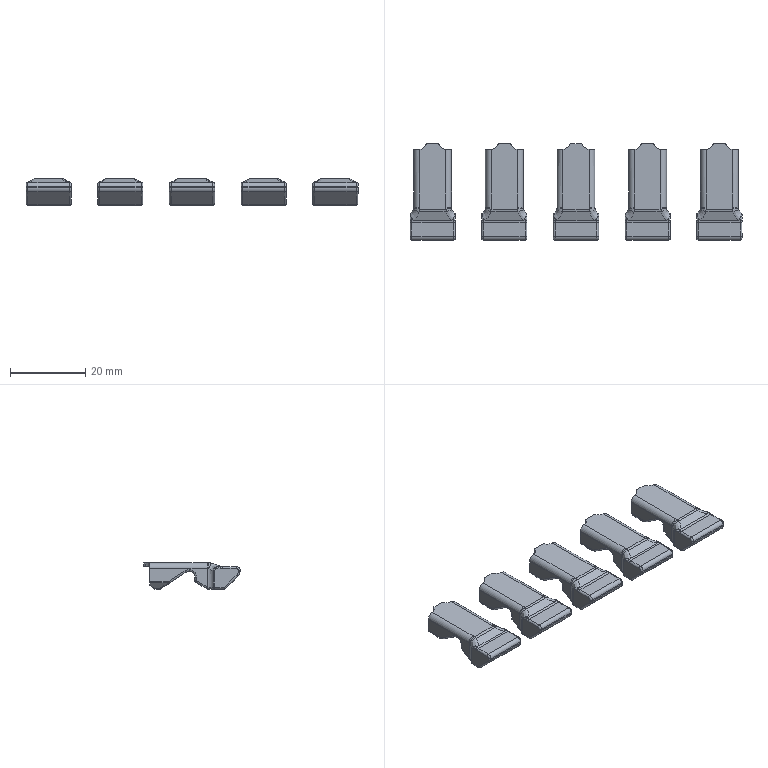NC program | NX | posted with a generic post | part box 88 x 25.5 x 7 mm
Lines 1 to 1151 of 11356:
N10 G17 G21 G94 G90
(FIXED_CONTOUR_COPY , TOOL : D4R0.5)
N12 T18 M6
N14 G54
N16 G17 G0 G90 X12.471 Y-7.984 S9500 M3
N18 G43 Z30. H18
N20 Z2.
N22 G94 G1 Z-2.898 F2500.
N24 X12.434 Y-7.987 Z-2.5
N26 X12.425 Z-2.401
N28 X12.353 Y-7.993 Z-2.4
N30 X12.313 Y-7.996 Z-2.305
N32 X12.265 Z-2.202
N34 X12.099 Z-2.032
N36 X12.03 Y-7.992 Z-1.974
N38 X11.941 Y-7.991 Z-1.95
N40 X11.702 Y-7.993 Z-1.909
N42 X8.531 Y-7.992 Z-1.899
N44 X7.995 Y-7.99 Z-1.883
N46 X7.831 Y-7.991 Z-1.878
N48 X7.738 Y-7.992 Z-1.869
N50 X7.342 Y-7.994 Z-1.807
N52 X7.216 Y-7.992 Z-1.79
N54 X6.945 Y-7.993 Z-1.788
N56 X6.828 Y-7.992 Z-1.808
N58 X6.549 Y-7.994 Z-1.891
N60 X6.318 Y-7.996 Z-2.026
N62 X6.139 Z-2.187
N64 X6.089 Y-7.995 Z-2.244
N66 X5.988 Y-7.993 Z-2.421
N68 X5.919 Y-7.99 Z-2.632
N70 X5.834 Y-7.987 Z-2.724
N72 Z-2.756
N74 X5.767 Y-7.984 Z-2.752
N76 X5.723 Y-7.979 Z-2.745
N78 X5.724 Z-2.721
N80 X5.756 Y-7.984 Z-2.651
N82 X5.761
N84 X5.827 Y-7.986 Z-2.584
N86 X5.875 Y-7.987 Z-2.447
N88 X5.992 Y-7.985 Z-2.214
N90 X6.153 Y-7.987 Z-2.039
N92 X6.218 Y-7.986 Z-1.981
N94 X6.337 Y-7.985 Z-1.899
N96 X6.4 Z-1.862
N98 X6.549 Y-7.983 Z-1.787
N100 X6.783 Y-7.981 Z-1.718
N102 X6.825 Y-7.98 Z-1.708
N104 X6.945 Y-7.981 Z-1.689
N106 X7.222 Z-1.69
N108 X7.354 Y-7.982 Z-1.709
N110 X7.751 Y-7.98 Z-1.77
N112 X7.995 Y-7.979 Z-1.793
N114 X8.135 Z-1.797
N116 X8.531 Y-7.98 Z-1.8
N118 X11.715 Y-7.981 Z-1.811
N120 X12.085 Y-7.983 Z-1.891
N122 X12.101 Y-7.984 Z-1.904
N124 X12.22 Y-7.987 Z-2.013
N126 X12.311 Z-2.107
N128 X12.407 Y-7.989 Z-2.271
N130 X12.487 Y-7.983 Z-2.322
N132 X12.495 Y-7.982 Z-2.33
N134 X12.521 Y-7.979 Z-2.479
N136 Z-2.5
N138 Z-2.479
N140 X12.516 Z-2.451
N142 X12.515 Z-2.298
N144 X12.495 Z-2.256
N146 X12.309 Z-1.988
N148 X12.114 Z-1.871
N150 X12.099 Z-1.864
N152 X11.702 Z-1.799
N154 X8.488
N156 X8.135 Z-1.797
N158 X7.995 Z-1.793
N160 X7.759 Z-1.769
N162 X7.738 Z-1.767
N164 X7.342 Z-1.687
N166 X6.945 Z-1.679
N168 X6.549 Z-1.759
N170 X6.338 Z-1.843
N172 X6.153 Z-1.953
N174 X6.134 Z-1.97
N176 X6.11 Z-1.995
N178 X5.911 Z-2.239
N180 X5.756 Z-2.486
N182 X5.729 Z-2.564
N184 X5.728 Z-2.712
N186 X5.724 Z-2.721
N188 X5.723 Z-2.745
N190 X5.656 Y-7.969 Z-2.735
N192 X5.661 Z-2.67
N194 X5.662 Z-2.565
N196 X5.756 Z-2.299
N198 X5.774 Z-2.27
N200 X5.797 Z-2.242
N202 X5.992 Z-2.029
N204 X6.153 Z-1.888
N206 X6.208 Z-1.854
N208 X6.34 Z-1.786
N210 X6.485 Z-1.735
N212 X6.549 Z-1.71
N214 X6.826 Z-1.661
N216 X6.945 Z-1.636
N218 X7.342 Z-1.647
N220 X7.738 Z-1.726
N222 X7.995 Z-1.757
N224 X8.135 Z-1.76
N226 X11.702
N228 X11.824 Z-1.78
N230 X12.099 Z-1.818
N232 X12.233 Z-1.877
N234 X12.308 Z-1.922
N236 X12.454 Z-2.045
N238 X12.495 Z-2.104
N240 X12.595 Z-2.315
N242 X12.596 Z-2.5
N244 X12.695 Y-7.956
N246 X12.694 Z-2.336
N248 X12.545 Z-2.058
N250 X12.495 Z-1.997
N252 X12.406 Z-1.922
N254 X12.334 Z-1.872
N256 X12.305 Z-1.855
N258 X12.144 Z-1.785
N260 X12.099 Z-1.769
N262 X12.007 Z-1.758
N264 X11.702 Z-1.716
N266 X8.135
N268 X7.995 Z-1.712
N270 X7.738 Z-1.68
N272 X7.342 Z-1.601
N274 X6.945 Z-1.591
N276 X6.549 Z-1.66
N278 X6.502 Z-1.674
N280 X6.342 Z-1.73
N282 X6.297 Z-1.75
N284 X6.153 Z-1.825
N286 X6.082 Z-1.875
N288 X5.898 Z-2.03
N290 X5.816 Z-2.103
N292 X5.756 Z-2.168
N294 X5.704 Z-2.261
N296 X5.601 Z-2.501
N298 X5.578 Z-2.566
N300 Z-2.588
N302 X5.568 Z-2.726
N304 X5.474 Y-7.935 Z-2.735
N306 X5.48 Z-2.583
N308 X5.561 Z-2.353
N310 X5.611 Z-2.236
N312 X5.639 Z-2.186
N314 X5.756 Z-2.042
N316 X5.895 Z-1.925
N318 X6.153 Z-1.742
N320 X6.18 Z-1.728
N322 X6.345 Z-1.656
N324 X6.549 Z-1.591
N326 X6.945 Z-1.527
N328 X7.342 Z-1.533
N330 X7.738 Z-1.61
N332 X7.995 Z-1.646
N334 X8.135 Z-1.649
N336 X11.702 Z-1.65
N338 X12.099 Z-1.698
N340 X12.265 Z-1.758
N342 X12.301 Z-1.774
N344 X12.424 Z-1.845
N346 X12.495 Z-1.895
N348 X12.548 Z-1.941
N350 X12.621 Z-2.018
N352 X12.648 Z-2.051
N354 X12.689 Z-2.128
N356 X12.757 Z-2.276
N358 X12.788 Z-2.36
N360 X12.789 Z-2.5
N362 X12.886 Y-7.914
N364 Z-2.385
N366 X12.82 Z-2.213
N368 X12.762 Z-2.083
N370 X12.733 Z-2.038
N372 X12.682 Z-1.973
N374 X12.626 Z-1.913
N376 X12.543 Z-1.842
N378 X12.495 Z-1.81
N380 X12.342 Z-1.729
N382 X12.297 Z-1.711
N384 X12.252 Z-1.699
N386 X12.099 Z-1.644
N388 X12. Z-1.635
N390 X11.702 Z-1.6
N392 X8.135 Y-7.913
N394 X7.995 Z-1.596
N396 X7.802 Z-1.569
N398 X7.342 Z-1.481
N400 X6.945 Z-1.476
N402 X6.648 Z-1.524
N404 X6.549 Z-1.538
N406 X6.397 Z-1.585
N408 X6.348 Z-1.598
N410 X6.297 Z-1.615
N412 X6.153 Z-1.678
N414 X6.063 Z-1.728
N416 X5.756 Z-1.94
N418 X5.743 Z-1.952
N420 X5.705 Z-1.99
N422 X5.567 Z-2.16
N424 X5.527 Z-2.22
N426 X5.506 Z-2.262
N428 X5.385 Z-2.603
N430 X5.383 Z-2.744
N432 X5.36 Y-7.908 Z-2.746
N434 X5.298 Y-7.888 Z-2.752
N436 Z-2.651
N438 X5.3 Z-2.622
N440 X5.36 Z-2.39
N442 X5.375 Z-2.347
N444 X5.443 Z-2.211
N446 X5.518 Z-2.099
N448 X5.549 Z-2.057
N450 X5.688 Z-1.912
N452 X5.756 Z-1.855
N454 X5.927 Z-1.736
N456 X6.153 Z-1.612
N458 X6.225 Z-1.581
N460 X6.352 Z-1.536
N462 X6.473 Z-1.505
N464 X6.549 Z-1.481
N466 X6.797 Z-1.447
N468 X6.945 Z-1.423
N470 X7.342 Z-1.428
N472 X7.59 Z-1.473
N474 X7.899 Z-1.531
N476 X7.995 Z-1.545
N478 X8.135 Z-1.549
N480 X11.702
N482 X11.851 Z-1.567
N484 X12.099 Z-1.588
N486 X12.175 Z-1.616
N488 X12.292 Z-1.648
N490 X12.408 Z-1.695
N492 X12.495 Z-1.741
N494 X12.56 Z-1.779
N496 X12.674 Z-1.859
N498 X12.707 Z-1.887
N500 X12.748 Z-1.93
N502 X12.818 Z-2.019
N504 X12.894 Z-2.142
N506 X12.968 Z-2.383
N508 X12.969 Z-2.5
N510 X13.064 Y-7.858
N512 X13.063 Z-2.379
N514 X13.044 Z-2.316
N516 X12.975 Z-2.122
N518 X12.923 Z-2.018
N520 X12.892 Z-1.975
N522 X12.788 Z-1.866
N524 X12.664 Z-1.763
N526 X12.624 Z-1.735
N528 X12.487 Z-1.655
N530 X12.287 Z-1.576
N532 X12.099 Z-1.525
N534 X11.702 Z-1.492
N536 X8.135 Z-1.491
N538 X7.995 Z-1.486
N540 X7.342 Z-1.369
N542 X6.945 Z-1.364
N544 X6.549 Z-1.418
N546 X6.357 Z-1.466
N548 X6.153 Z-1.537
N550 X6.126 Z-1.55
N552 X5.768 Z-1.745
N554 X5.756 Z-1.753
N556 X5.624 Z-1.865
N558 X5.582 Z-1.909
N560 X5.468 Z-2.033
N562 X5.36 Z-2.182
N564 X5.342 Z-2.212
N566 X5.286 Z-2.343
N568 X5.209 Z-2.642
N570 X5.204 Z-2.717
N572 Z-2.762
N574 X5.137 Y-7.837 Z-2.763
N576 X5.109 Y-7.825
N578 X5.114 Z-2.656
N580 X5.142 Z-2.533
N582 X5.196 Z-2.326
N584 X5.215 Z-2.282
N586 X5.268 Z-2.18
N588 X5.36 Z-2.033
N590 X5.379 Z-2.006
N592 X5.433 Z-1.948
N594 X5.556 Z-1.828
N596 X5.591 Z-1.796
N598 X5.69 Z-1.72
N600 X5.756 Z-1.674
N602 X5.941 Z-1.573
N604 X6.153 Y-7.826 Z-1.476
N606 X6.272 Z-1.439
N608 X6.362 Z-1.408
N610 X6.464 Z-1.386
N612 X6.549 Z-1.364
N614 X6.771 Z-1.339
N616 X6.945 Z-1.315
N618 X7.342 Z-1.321
N620 X7.516 Z-1.352
N622 X7.738 Z-1.384
N624 X7.995 Z-1.434
N626 X8.073 Z-1.44
N628 X8.135 Z-1.442
N630 X11.702
N632 X11.877 Z-1.457
N634 X12.099 Z-1.472
N636 X12.183 Z-1.496
N638 X12.28 Z-1.516
N640 X12.385 Z-1.556
N642 X12.495 Z-1.591
N644 X12.557 Z-1.622
N646 X12.653 Z-1.673
N648 X12.693 Z-1.699
N650 X12.838 Z-1.811
N652 X12.878 Z-1.844
N654 X12.892 Z-1.858
N656 X12.985 Z-1.977
N658 X13.054 Z-2.08
N660 X13.064 Z-2.1
N662 X13.088 Z-2.168
N664 X13.141 Z-2.34
N666 X13.153 Z-2.384
N668 Z-2.5
N670 X13.246 Y-7.788
N672 Z-2.397
N674 X13.214 Z-2.278
N676 X13.173 Z-2.147
N678 X13.152 Z-2.096
N680 X13.071 Z-1.953
N682 X12.945 Z-1.81
N684 X12.892 Z-1.766
N686 X12.769 Z-1.672
N688 X12.634 Z-1.586
N690 X12.495 Z-1.519
N692 X12.273 Z-1.451
N694 X12.099 Z-1.416
N696 X11.702 Z-1.388
N698 X8.135
N700 X8. Z-1.379
N702 X7.738 Z-1.325
N704 X7.342 Z-1.268
N706 X6.945 Z-1.261
N708 X6.549 Z-1.307
N710 X6.341 Z-1.353
N712 X6.13 Z-1.418
N714 X5.756 Z-1.59
N716 X5.609 Z-1.688
N718 X5.48 Z-1.804
N720 X5.326 Z-1.953
N722 X5.302 Z-1.982
N724 X5.196 Z-2.128
N726 X5.177 Z-2.158
N728 X5.16 Z-2.192
N730 X5.102 Z-2.322
N732 X5.065 Z-2.466
N734 X5.023 Z-2.649
N736 X5.021 Z-2.763
N738 X4.931 Y-7.749
N740 X4.932 Z-2.666
N742 X4.948 Z-2.569
N744 X4.963 Z-2.515
N746 X5.011 Z-2.332
N748 X5.089 Z-2.157
N750 X5.162 Z-2.044
N752 X5.178 Z-2.025
N754 X5.226 Z-1.959
N756 X5.283 Z-1.891
N758 X5.401 Z-1.779
N760 X5.51 Z-1.681
N762 X5.612 Z-1.611
N764 X5.701 Z-1.561
N766 X5.756 Z-1.525
N768 X6.014 Z-1.405
N770 X6.153 Z-1.356
N772 X6.355 Z-1.298
N774 X6.549 Z-1.259
N776 X6.945 Z-1.216
N778 X7.342 Z-1.22
N780 X7.738 Z-1.274
N782 X8.025 Z-1.335
N784 X8.135 Z-1.341
N786 X11.702
N788 X12.099 Z-1.368
N790 X12.266 Z-1.398
N792 X12.428 Z-1.446
N794 X12.495 Z-1.466
N796 X12.58 Z-1.497
N798 X12.674 Z-1.541
N800 X12.801 Z-1.613
N802 X12.85 Z-1.644
N804 X13.01 Z-1.773
N806 X13.083 Z-1.854
N808 X13.149 Z-1.933
N810 X13.18 Z-1.984
N812 X13.242 Z-2.098
N814 X13.291 Z-2.217
N816 X13.322 Z-2.345
N818 X13.334 Z-2.42
N820 Z-2.5
N822 X13.375 Y-7.729
N824 X13.419 Y-7.705
N826 Z-2.424
N828 X13.402 Z-2.317
N830 X13.391 Z-2.27
N832 X13.374 Z-2.213
N834 X13.34 Z-2.119
N836 X13.288 Z-2.01
N838 X13.247 Z-1.934
N840 X13.133 Z-1.791
N842 X13.109 Z-1.767
N844 X13.069 Z-1.732
N846 X12.954 Z-1.638
N848 X12.892 Z-1.594
N850 X12.742 Z-1.51
N852 X12.653 Z-1.469
N854 X12.543 Z-1.431
N856 X12.495 Z-1.411
N858 X12.355 Z-1.369
N860 X12.306 Z-1.357
N862 X12.249 Z-1.348
N864 X12.222 Z-1.342
N866 X12.099 Z-1.32
N868 X11.702 Z-1.294
N870 X8.098 Z-1.293
N872 X8.044 Z-1.288
N874 X7.738 Z-1.224
N876 X7.342 Z-1.172
N878 X6.945 Z-1.169
N880 X6.549 Z-1.209
N882 X6.302 Z-1.259
N884 X6.153 Z-1.3
N886 X5.906 Z-1.388
N888 X5.756 Z-1.458
N890 X5.554 Z-1.574
N892 X5.435 Z-1.655
N894 X5.294 Z-1.781
N896 X5.217 Z-1.866
N898 X5.166 Z-1.914
N900 X5.115 Z-1.974
N902 X5.004 Z-2.146
N904 X4.924 Z-2.33
N906 X4.885 Z-2.459
N908 X4.847 Z-2.688
N910 X4.844 Z-2.763
N912 X4.761 Y-7.657
N914 X4.765 Z-2.671
N916 X4.805 Z-2.447
N918 X4.845 Z-2.314
N920 X4.927 Z-2.129
N922 X5.02 Z-1.978
N924 X5.078 Z-1.906
N926 X5.165 Z-1.811
N928 X5.387 Z-1.61
N930 X5.431 Z-1.581
N932 X5.756 Z-1.394
N934 X5.811 Z-1.368
N936 X6.009 Z-1.301
N938 X6.153 Z-1.247
N940 X6.207 Z-1.232
N942 X6.549 Z-1.162
N944 X6.945 Z-1.124
N946 X7.342 Z-1.128
N948 X7.451 Z-1.142
N950 X7.738 Z-1.177
N952 X8.056 Z-1.241
N954 X8.1 Z-1.248
N956 X8.531 Z-1.251
N958 X11.702
N960 X12.099 Z-1.276
N962 X12.157 Z-1.287
N964 X12.3 Z-1.305
N966 X12.444 Z-1.34
N968 X12.495 Z-1.356
N970 X12.639 Z-1.414
N972 X12.718 Z-1.442
N974 X12.837 Z-1.494
N976 X12.892 Z-1.525
N978 X13.078 Z-1.654
N980 X13.165 Z-1.728
N982 X13.227 Z-1.789
N984 X13.288 Z-1.863
N986 X13.325 Z-1.913
N988 X13.35 Z-1.956
N990 X13.373 Z-2.013
N992 X13.442 Z-2.157
N994 X13.465 Z-2.226
N996 X13.499 Z-2.368
N998 X13.504 Z-2.4
N1000 Z-2.5
N1002 X13.555 Y-7.628
N1004 X13.585 Y-7.608
N1006 Z-2.392
N1008 X13.544 Z-2.198
N1010 X13.522 Z-2.132
N1012 X13.486 Z-2.046
N1014 X13.406 Z-1.909
N1016 X13.349 Z-1.832
N1018 X13.309 Z-1.783
N1020 X13.179 Z-1.655
N1022 X13.136 Z-1.622
N1024 X12.935 Z-1.483
N1026 X12.892 Z-1.46
N1028 X12.786 Z-1.414
N1030 X12.737 Z-1.397
N1032 X12.582 Z-1.334
N1034 X12.495 Z-1.305
N1036 X12.449 Z-1.296
N1038 X12.294 Z-1.258
N1040 X12.099 Z-1.233
N1042 X11.702 Z-1.21
N1044 X8.135 Z-1.209
N1046 X8.118 Z-1.208
N1048 X7.738 Z-1.132
N1050 X7.651 Z-1.124
N1052 X7.342 Z-1.087
N1054 X6.945 Z-1.083
N1056 X6.549 Z-1.118
N1058 X6.24 Z-1.182
N1060 X6.153 Z-1.197
N1062 X6.066 Z-1.225
N1064 X5.911 Z-1.283
N1066 X5.756 Z-1.334
N1068 X5.669 Z-1.377
N1070 X5.36 Z-1.555
N1072 X5.311 Z-1.59
N1074 X5.063 Z-1.817
N1076 X4.94 Z-1.97
N1078 X4.904 Z-2.023
N1080 X4.847 Z-2.118
N1082 X4.765 Z-2.298
N1084 X4.724 Z-2.438
N1086 X4.684 Z-2.669
N1088 X4.681 Z-2.763
N1090 X4.597 Y-7.554
N1092 X4.6 Z-2.685
N1094 X4.639 Z-2.447
N1096 X4.679 Z-2.304
N1098 X4.759 Z-2.109
N1100 X4.883 Z-1.928
N1102 X4.993 Z-1.787
N1104 X5.19 Z-1.604
N1106 X5.293 Z-1.536
N1108 X5.36 Z-1.482
N1110 X5.452 Z-1.429
N1112 X5.756 Z-1.278
N1114 X5.849 Z-1.245
N1116 X6.001 Z-1.199
N1118 X6.153 Z-1.149
N1120 X6.456 Z-1.095
N1122 X6.549 Z-1.076
N1124 X6.945 Z-1.044
N1126 X7.342 Z-1.048
N1128 X7.435 Z-1.059
N1130 X7.738 Z-1.088
N1132 X8.145 Z-1.168
N1134 X8.531 Z-1.17
N1136 X11.702
N1138 X12.099 Z-1.191
N1140 X12.288 Z-1.213
N1142 X12.334 Z-1.224
N1144 X12.495 Z-1.258
N1146 X12.799 Z-1.359
N1148 X12.892 Z-1.397
N1150 X13.043 Z-1.477
N1152 X13.104 Z-1.519
N1154 X13.255 Z-1.634
N1156 X13.362 Z-1.741
N1158 X13.493 Z-1.902
N1160 X13.584 Z-2.08
N1162 X13.642 Z-2.254
N1164 X13.664 Z-2.366
N1166 X13.669 Z-2.395
N1168 Z-2.5
N1170 X13.684 Y-7.544
N1172 X13.742 Y-7.498
N1174 Z-2.403
N1176 X13.723 Z-2.268
N1178 X13.684 Z-2.132
N1180 X13.674 Z-2.1
N1182 X13.588 Z-1.931
N1184 X13.557 Z-1.879
N1186 X13.417 Z-1.697
N1188 X13.389 Z-1.669
N1190 X13.288 Z-1.581
N1192 X13.156 Z-1.481
N1194 X13.07 Z-1.432
N1196 X12.938 Z-1.362
N1198 X12.892 Z-1.34
N1200 X12.628 Z-1.252
N1202 X12.495 Z-1.214
N1204 X12.355 Z-1.185
N1206 X12.281 Z-1.174
N1208 X12.099 Z-1.155
N1210 X11.702 Z-1.135
N1212 X8.283
N1214 X8.177 Z-1.136
N1216 X8.074 Z-1.114
N1218 X7.738 Z-1.05
N1220 X7.342 Z-1.013
N1222 X6.945 Z-1.009
N1224 X6.549 Z-1.039
N1226 X6.286 Z-1.086
N1228 X6.153 Z-1.107
N1230 X6.02 Z-1.143
N1232 X5.888 Z-1.187
N1234 X5.756 Z-1.227
N1236 X5.623 Z-1.287
N1238 X5.36 Z-1.417
N1240 X5.301 Z-1.453
N1242 X5.243 Z-1.499
N1244 X5.154 Z-1.559
N1246 X5.079 Z-1.617
N1248 X4.933 Z-1.756
N1250 X4.855 Y-7.497 Z-1.842
N1252 X4.823 Z-1.884
N1254 X4.799 Z-1.919
N1256 X4.67 Z-2.134
N1258 X4.59 Z-2.317
N1260 X4.567 Z-2.399
N1262 X4.553 Z-2.46
N1264 X4.524 Z-2.689
N1266 X4.522 Z-2.763
N1268 X4.446 Y-7.436
N1270 X4.448 Z-2.687
N1272 X4.455 Z-2.612
N1274 X4.472 Z-2.486
N1276 X4.509 Z-2.328
N1278 X4.571 Z-2.162
N1280 X4.732 Z-1.895
N1282 X4.763 Z-1.852
N1284 X4.833 Z-1.767
N1286 X4.875 Z-1.721
N1288 X4.97 Z-1.629
N1290 X5.192 Z-1.456
N1292 X5.36 Z-1.354
N1294 X5.661 Z-1.217
N1296 X5.756 Z-1.176
N1298 X6.057 Z-1.09
N1300 X6.153 Z-1.066
N1302 X6.549 Z-1.002
N1304 X6.945 Z-0.975
N1306 X7.342 Z-0.977
N1308 X7.738 Z-1.013
N1310 X8.135 Z-1.087
N1312 X8.211 Z-1.107
N1314 X8.516 Z-1.102
N1316 X11.702
N1318 X12.099 Z-1.121
N1320 X12.273 Z-1.138
N1322 X12.495 Z-1.171
N1324 X12.892 Z-1.285
N1326 X13.033 Z-1.352
N1328 X13.185 Z-1.437
N1330 X13.288 Z-1.5
N1332 X13.394 Z-1.591
N1334 X13.48 Z-1.67
N1336 X13.555 Z-1.759
N1338 X13.627 Z-1.853
N1340 X13.687 Z-1.955
N1342 X13.753 Z-2.105
N1344 X13.794 Z-2.25
N1346 X13.819 Z-2.413
N1348 Z-2.5
N1350 X13.897 Y-7.373
N1352 X13.896 Z-2.415
N1354 X13.867 Z-2.231
N1356 X13.831 Z-2.109
N1358 X13.765 Z-1.957
N1360 X13.7 Z-1.834
N1362 X13.544 Z-1.647
N1364 X13.471 Z-1.584
N1366 X13.426 Z-1.542
N1368 X13.306 Z-1.448
N1370 X13.247 Z-1.412
N1372 X13.066 Z-1.313
N1374 X12.996 Z-1.284
N1376 X12.939 Z-1.258
N1378 X12.774 Z-1.208
N1380 X12.612 Z-1.162
N1382 X12.495 Z-1.136
N1384 X12.265 Z-1.105
N1386 X12.099 Z-1.09
N1388 X11.937 Z-1.083
N1390 X11.702 Z-1.075
N1392 X8.375
N1394 X8.245 Z-1.078
N1396 X8.135 Z-1.05
N1398 X8.049 Z-1.032
N1400 X7.856 Z-0.997
N1402 X7.738 Z-0.982
N1404 X7.577 Z-0.967
N1406 X7.342 Z-0.95
N1408 X6.945 Z-0.947
N1410 X6.711 Z-0.961
N1412 X6.549 Z-0.972
N1414 X6.432 Z-0.985
N1416 X6.153 Z-1.03
N1418 X6.035 Z-1.055
N1420 X5.756 Z-1.133
N1422 X5.639 Z-1.174
N1424 X5.36 Z-1.3
N1426 X5.284 Z-1.341
N1428 X5.171 Z-1.409
N1430 X5.054 Z-1.491
N1432 X4.963 Z-1.561
N1434 X4.921 Z-1.597
N1436 X4.81 Z-1.7
N1438 X4.704 Z-1.825
N1440 X4.632 Z-1.926
N1442 X4.567 Z-2.033
N1444 X4.494 Z-2.171
N1446 X4.432 Z-2.338
N1448 X4.39 Z-2.512
N1450 X4.371 Z-2.686
N1452 X4.369 Z-2.763
N1454 X4.32 Y-7.333
N1456 X4.295 Y-7.308
N1458 X4.297 Z-2.687
N1460 X4.314 Z-2.525
N1462 X4.363 Z-2.331
N1464 X4.423 Z-2.167
N1466 X4.549 Z-1.932
N1468 X4.642 Z-1.802
N1470 X4.741 Z-1.69
N1472 X4.827 Z-1.606
N1474 X4.876 Z-1.563
N1476 X4.963 Z-1.49
N1478 X5.038 Z-1.437
N1480 X5.137 Z-1.371
N1482 X5.199 Z-1.335
N1484 X5.348 Z-1.254
N1486 X5.546 Z-1.166
N1488 X5.732 Z-1.1
N1490 X5.93 Z-1.044
N1492 X6.153 Z-0.998
N1494 X6.326 Z-0.97
N1496 X6.549 Z-0.944
N1498 X6.889 Z-0.926
N1500 X7.043 Z-0.924
N1502 X7.342 Z-0.926
N1504 X7.738 Z-0.954
N1506 X8.008 Z-0.989
N1508 X8.178 Z-1.025
N1510 X8.291 Z-1.052
N1512 X11.754 Z-1.053
N1514 X12.125 Z-1.066
N1516 X12.381 Z-1.09
N1518 X12.553 Z-1.114
N1520 X12.702 Z-1.147
N1522 X12.892 Z-1.204
N1524 X12.998 Z-1.238
N1526 X13.139 Z-1.298
N1528 X13.288 Z-1.378
N1530 X13.339 Z-1.409
N1532 X13.509 Z-1.54
N1534 X13.607 Z-1.626
N1536 X13.714 Z-1.755
N1538 X13.771 Z-1.83
N1540 X13.837 Z-1.951
N1542 X13.852 Z-1.983
N1544 X13.904 Z-2.103
N1546 X13.938 Z-2.213
N1548 X13.95 Z-2.281
N1550 X13.972 Z-2.419
N1552 X13.973 Z-2.5
N1554 X14.044 Y-7.238
N1556 X14.042 Z-2.412
N1558 X14.035 Z-2.36
N1560 X14.005 Z-2.197
N1562 X13.969 Z-2.08
N1564 X13.899 Z-1.933
N1566 X13.831 Z-1.811
N1568 X13.679 Z-1.619
N1570 X13.568 Z-1.516
N1572 X13.397 Z-1.389
N1574 X13.279 Z-1.319
N1576 X13.184 Z-1.274
N1578 X13.072 Z-1.228
N1580 X13.018 Z-1.211
N1582 X12.892 Z-1.167
N1584 X12.719 Z-1.114
N1586 X12.59 Z-1.094
N1588 X12.41 Z-1.069
N1590 X12.2 Z-1.051
N1592 X12.099 Z-1.044
N1594 X11.903 Z-1.038
N1596 X11.426 Z-1.033
N1598 X8.927
N1600 X8.527 Z-1.031
N1602 X8.466 Z-1.033
N1604 X8.359
N1606 X8.302 Z-1.02
N1608 X8.214 Z-1.005
N1610 X8.059 Z-0.971
N1612 X7.964 Z-0.958
N1614 X7.87 Z-0.95
N1616 X7.738 Z-0.933
N1618 X7.324 Z-0.905
N1620 X7.134 Z-0.907
N1622 X6.945 Z-0.906
N1624 X6.729 Z-0.913
N1626 X6.549 Z-0.921
N1628 X6.256 Z-0.954
N1630 X6.153 Z-0.971
N1632 X5.964 Z-1.007
N1634 X5.86 Z-1.029
N1636 X5.662 Z-1.085
N1638 X5.511 Z-1.138
N1640 X5.463 Z-1.156
N1642 X5.313 Z-1.223
N1644 X5.218 Z-1.271
N1646 X5.171 Z-1.3
N1648 X5.067 Z-1.358
N1650 X4.963 Z-1.422
N1652 X4.797 Z-1.558
N1654 X4.671 Z-1.679
N1656 X4.567 Z-1.793
N1658 X4.52 Z-1.867
N1660 X4.473 Z-1.932
N1662 X4.361 Z-2.141
N1664 X4.305 Z-2.291
N1666 X4.282 Z-2.371
N1668 X4.247 Z-2.514
N1670 X4.227 Z-2.693
N1672 X4.226 Z-2.763
N1674 X4.158 Y-7.167
N1676 Z-2.697
N1678 X4.179 Z-2.502
N1680 X4.205 Z-2.39
N1682 X4.247 Z-2.251
N1684 X4.298 Z-2.115
N1686 X4.338 Z-2.038
N1688 X4.403 Z-1.921
N1690 X4.448 Z-1.855
N1692 X4.484 Z-1.808
N1694 X4.5 Z-1.783
N1696 X4.55 Z-1.721
N1698 X4.615 Z-1.652
N1700 X4.726 Z-1.546
N1702 X4.83 Z-1.459
N1704 X4.93 Z-1.385
N1706 X5.111 Z-1.275
N1708 X5.194 Z-1.232
N1710 X5.277 Z-1.191
N1712 X5.392 Z-1.142
N1714 X5.507 Z-1.098
N1716 X5.59 Z-1.07
N1718 X5.789 Z-1.014
N1720 X5.987 Z-0.973
N1722 X6.07 Z-0.96
N1724 X6.185 Z-0.938
N1726 X6.549 Z-0.901
N1728 X6.945 Z-0.889
N1730 X7.342
N1732 X7.673 Z-0.906
N1734 X7.771 Z-0.914
N1736 X7.945 Z-0.93
N1738 X8.111 Z-0.953
N1740 X8.274 Z-0.989
N1742 X8.429 Z-1.015
N1744 X8.531 Z-1.016
N1746 X8.927 Z-1.014
N1748 X11.306
N1750 X11.702 Z-1.019
N1752 X12.099 Z-1.023
N1754 X12.324 Z-1.039
N1756 X12.474 Z-1.054
N1758 X12.705 Z-1.086
N1760 X12.839 Z-1.113
N1762 X12.892 Z-1.13
N1764 X13.148 Z-1.217
N1766 X13.256 Z-1.262
N1768 X13.288 Z-1.277
N1770 X13.42 Z-1.348
N1772 X13.457 Z-1.37
N1774 X13.65 Z-1.517
N1776 X13.684 Z-1.549
N1778 X13.781 Z-1.654
N1780 X13.892 Z-1.792
N1782 X13.965 Z-1.924
N1784 X14.019 Z-2.038
N1786 X14.044 Z-2.11
N1788 X14.08 Z-2.227
N1790 X14.107 Z-2.431
N1792 Z-2.5
N1794 X14.162 Y-7.098
N1796 Z-2.434
N1798 X14.136 Z-2.225
N1800 X14.109 Z-2.133
N1802 X14.062 Z-1.991
N1804 X14.045 Z-1.956
N1806 X13.994 Z-1.87
N1808 X13.949 Z-1.783
N1810 X13.88 Z-1.688
N1812 X13.724 Z-1.519
N1814 X13.52 Z-1.362
N1816 X13.448 Z-1.32
N1818 X13.288 Z-1.235
N1820 X13.221 Z-1.207
N1822 X12.964 Z-1.121
N1824 X12.892 Z-1.101
N1826 X12.73 Z-1.068
N1828 X12.555 Z-1.044
N1830 X12.394 Z-1.032
N1832 X12.314 Z-1.022
N1834 X12.267 Z-1.023
N1836 X12.099 Z-1.013
N1838 X11.66 Z-1.007
N1840 X8.505
N1842 X8.395 Z-0.984
N1844 X8.332 Z-0.973
N1846 X8.238 Z-0.953
N1848 X8.167 Z-0.94
N1850 X7.927 Z-0.908
N1852 X7.738 Z-0.894
N1854 X7.342 Z-0.875
N1856 X7.018 Z-0.874
N1858 X6.945 Z-0.872
N1860 X6.549 Z-0.884
N1862 X6.347 Z-0.904
N1864 X6.153 Z-0.919
N1866 X6.116 Z-0.924
N1868 X6.035 Z-0.94
N1870 X5.918 Z-0.958
N1872 X5.756 Z-0.992
N1874 X5.594 Z-1.038
N1876 X5.558 Z-1.046
N1878 X5.422 Z-1.091
N1880 X5.219 Z-1.174
N1882 X5.139 Z-1.214
N1884 X5.108 Z-1.231
N1886 X5.026 Z-1.27
N1888 X4.95 Z-1.319
N1890 X4.932 Z-1.329
N1892 X4.733 Z-1.468
N1894 X4.641 Z-1.545
N1896 X4.56 Z-1.619
N1898 X4.534 Z-1.65
N1900 X4.475 Z-1.709
N1902 X4.438 Z-1.752
N1904 X4.359 Z-1.858
N1906 X4.331 Z-1.902
N1908 X4.29 Z-1.981
N1910 X4.263 Z-2.048
N1912 X4.202 Z-2.173
N1914 X4.171 Z-2.274
N1916 X4.129 Z-2.445
N1918 X4.112 Z-2.544
N1920 X4.099 Z-2.692
N1922 X4.097 Z-2.763
N1924 X4.058 Y-7.05
N1926 Z-2.718
N1928 X4.066 Z-2.58
N1930 X4.085 Z-2.411
N1932 X4.119 Z-2.213
N1934 X4.139 Z-2.156
N1936 X4.171 Z-2.042
N1938 X4.207 Z-1.951
N1940 X4.348 Z-1.737
N1942 X4.364 Z-1.717
N1944 X4.402 Z-1.682
N1946 X4.417 Z-1.662
N1948 X4.476 Z-1.607
N1950 X4.526 Z-1.568
N1952 X4.541 Z-1.553
N1954 X4.697 Z-1.444
N1956 X4.742 Z-1.407
N1958 X4.893 Z-1.318
N1960 X4.978 Z-1.261
N1962 X5.181 Z-1.162
N1964 X5.374 Z-1.084
N1966 X5.558 Z-1.023
N1968 X5.643 Z-1.004
N1970 X5.756 Z-0.972
N1972 X5.87 Z-0.948
N1974 X6.011 Z-0.926
N1976 X6.068 Z-0.915
N1978 X6.153 Z-0.904
N1980 X6.549 Z-0.873
N1982 X6.945 Z-0.861
N1984 X7.115 Z-0.866
N1986 X7.342 Z-0.867
N1988 X7.885 Z-0.895
N1990 X8.211 Z-0.934
N1992 X8.37 Z-0.962
N1994 X8.563 Z-1.004
N1996 X11.306
N1998 X11.603 Z-1.003
N2000 X11.702 Z-1.006
N2002 X11.894
N2004 X12.099 Z-1.008
N2006 X12.257 Z-1.016
N2008 X12.319 Z-1.014
N2010 X12.374 Z-1.023
N2012 X12.445 Z-1.026
N2014 X12.633 Z-1.041
N2016 X12.721 Z-1.055
N2018 X12.778 Z-1.062
N2020 X12.892 Z-1.085
N2022 X12.976 Z-1.106
N2024 X13.23 Z-1.186
N2026 X13.288 Z-1.207
N2028 X13.401 Z-1.265
N2030 X13.485 Z-1.313
N2032 X13.569 Z-1.363
N2034 X13.775 Z-1.524
N2036 X13.838 Z-1.592
N2038 X13.911 Z-1.676
N2040 X13.988 Z-1.781
N2042 X14.02 Z-1.841
N2044 X14.095 Z-1.97
N2046 X14.159 Z-2.171
N2048 X14.175 Z-2.225
N2050 X14.201 Z-2.435
N2052 X14.202 Z-2.5
N2054 X14.226 Y-7.02
N2056 X14.225 Z-2.436
N2058 X14.199 Z-2.225
N2060 X14.172 Z-2.134
N2062 X14.119 Z-1.971
N2064 X14.081 Z-1.9
N2066 X14.036 Z-1.824
N2068 X14.012 Z-1.779
N2070 X13.929 Z-1.668
N2072 X13.807 Z-1.527
N2074 X13.599 Z-1.364
N2076 X13.485 Z-1.296
N2078 X13.402 Z-1.249
N2080 X13.288 Z-1.192
N2082 X13.006 Z-1.103
N2084 X12.892 Z-1.076
N2086 X12.808 Z-1.059
N2088 X12.73 Z-1.049
N2090 X12.672 Z-1.039
N2092 X12.458 Z-1.022
N2094 X12.362 Z-1.017
N2096 X12.321 Z-1.01
N2098 X12.238 Z-1.012
N2100 X12.099 Z-1.006
N2102 X11.961 Z-1.004
N2104 X11.702 Z-1.005
N2106 X11.604 Z-1.001
N2108 X8.826
N2110 X8.601 Z-1.003
N2112 X8.355 Z-0.951
N2114 X8.237 Z-0.931
N2116 X7.914 Z-0.892
N2118 X7.342 Z-0.862
N2120 X7.174 Z-0.861
N2122 X6.945 Z-0.855
N2124 X6.549 Z-0.865
N2126 X6.421 Z-0.873
N2128 X6.153 Z-0.894
N2130 X6.038 Z-0.909
N2132 X5.996 Z-0.918
N2134 X5.84 Z-0.942
N2136 X5.756 Z-0.959
N2138 X5.672 Z-0.983
N2140 X5.558 Z-1.009
N2142 X5.39 Z-1.064
N2144 X5.339 Z-1.079
N2146 X5.183 Z-1.141
N2148 X4.984 Z-1.236
N2150 X4.963 Z-1.243
N2152 X4.783 Z-1.349
N2154 X4.753 Z-1.36
N2156 X4.597 Z-1.467
N2158 X4.567 Z-1.48
N2160 X4.537 Z-1.5
N2162 X4.515 Z-1.51
N2164 X4.466 Z-1.548
N2166 X4.449 Z-1.558
N2168 X4.412 Z-1.591
N2170 X4.396 Z-1.598
N2172 X4.359 Z-1.632
N2174 X4.182 Z-1.816
N2176 X4.171 Z-1.833
N2178 X4.113 Z-1.933
N2180 X4.095 Z-2.018
N2182 X4.072 Z-2.15
N2184 X4.064 Z-2.213
N2186 X4.06 Z-2.304
N2188 X4.047 Z-2.389
N2190 X4.045 Z-2.479
N2192 X4.033 Z-2.688
N2194 Z-2.763
N2196 X4.022 Y-7.006
N2198 X4.02 Y-7.004 Z-2.449
N2200 X4.019 Y-7.003
N2202 X4.015 Z-2.
N2204 X3.975 Y-7.
N2206 X0.999 Y-6.997
N2208 X-2.965 Y-6.999
N2210 X-11.164 Y-6.998
N2212 X-11.25 Y-6.996 Z-1.922
N2214 Y-6.995 Z-1.913
N2216 X-10.893 Z-1.908
N2218 X3.975 Z-1.91
N2220 X3.985 Y-6.996 Z-1.903
N2222 X4.02 Y-6.998
N2224 X4.054 Y-7. Z-1.838
N2226 X4.095 Y-6.996 Z-1.771
N2228 X4.171 Y-6.995 Z-1.69
N2230 X4.314 Z-1.598
N2232 X4.378 Z-1.532
N2234 X4.421 Z-1.514
N2236 X4.431 Z-1.504
N2238 X4.475 Z-1.48
N2240 X4.488 Z-1.469
N2242 X4.56 Z-1.436
N2244 X4.567 Z-1.431
N2246 X4.647 Z-1.399
N2248 X4.757 Z-1.323
N2250 X4.837 Z-1.292
N2252 X4.963 Z-1.218
N2254 X5.044 Z-1.189
N2256 X5.176 Z-1.124
N2258 X5.306 Z-1.074
N2260 X5.44 Z-1.036
N2262 X5.558 Z-0.998
N2264 X5.697 Z-0.966
N2266 X5.756 Z-0.949
N2268 X5.815 Z-0.937
N2270 X5.984 Z-0.911
N2272 X6.013 Z-0.905
N2274 X6.153 Z-0.886
N2276 X6.342 Z-0.871
N2278 X6.549 Z-0.859
N2280 X6.945 Z-0.849
N2282 X7.224 Z-0.857
N2284 X7.342
N2286 X7.921 Z-0.888
N2288 X8.001 Z-0.896
N2290 X8.259 Z-0.927
N2292 X8.352 Z-0.943
N2294 X8.633 Z-1.002
N2296 X8.907 Z-1.
N2298 X11.633 Z-1.001
N2300 X11.702 Z-1.003